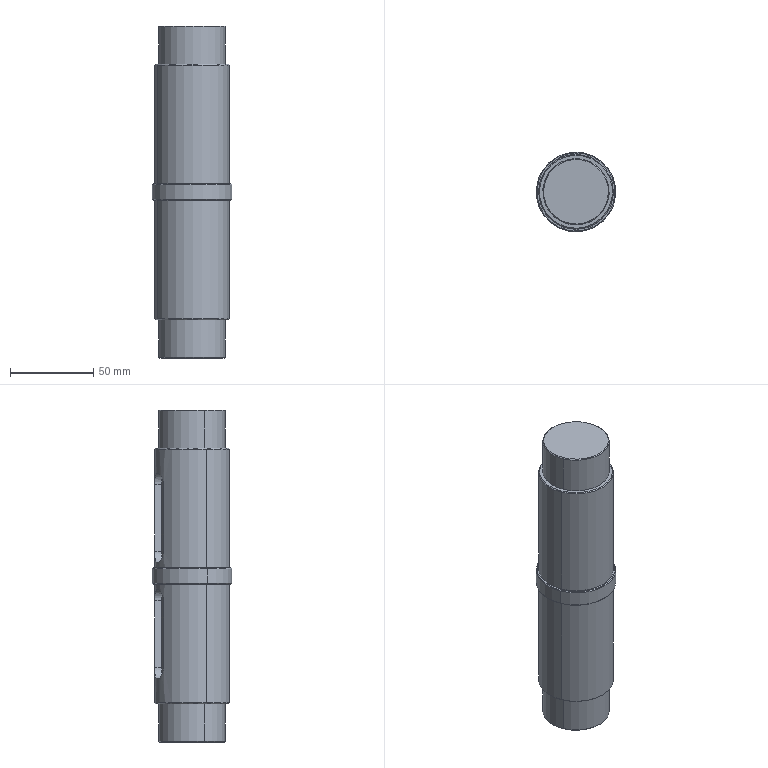Part | SolidWorks | features BaseBody 1 | 1 solid | 40 faces | box 48 x 48 x 200 mm | volume 297463 mm3 | cylinder 16 | cone 12 | plane 12 | commonest cylinder face diameters 14 x6 40 x4 45 x4 48 x2
STEP:
#1=CARTESIAN_POINT('',(446.784,55.988,-196.693));
#2=VERTEX_POINT('',#1);
#3=CARTESIAN_POINT('',(453.254,58.66,-203.693));
#4=VERTEX_POINT('',#3);
#5=CARTESIAN_POINT('',(446.784,55.988,-203.693));
#6=DIRECTION('',(-0.3818,0.9243,0.));
#7=DIRECTION('',(0.,0.,1.));
#8=AXIS2_PLACEMENT_3D('',#5,#6,#7);
#9=CIRCLE('',#8,7.);
#10=EDGE_CURVE('',#2,#4,#9,.T.);
#11=ORIENTED_EDGE('',*,*,#10,.F.);
#12=CARTESIAN_POINT('',(444.684,61.071,-196.693));
#13=VERTEX_POINT('',#12);
#14=CARTESIAN_POINT('',(446.784,55.988,-196.693));
#15=DIRECTION('',(-0.3818,0.9243,0.));
#16=VECTOR('',#15,1000.);
#17=LINE('',#14,#16);
#18=EDGE_CURVE('',#2,#13,#17,.T.);
#19=ORIENTED_EDGE('',*,*,#18,.T.);
#20=CARTESIAN_POINT('',(451.581,62.712,-203.693));
#21=VERTEX_POINT('',#20);
#22=CARTESIAN_POINT('',(451.581,62.712,-203.693));
#23=CARTESIAN_POINT('',(451.581,62.712,-203.227));
#24=CARTESIAN_POINT('',(451.532,62.708,-202.77));
#25=CARTESIAN_POINT('',(451.391,62.697,-202.096));
#26=CARTESIAN_POINT('',(451.333,62.692,-201.873));
#27=CARTESIAN_POINT('',(451.192,62.679,-201.432));
#28=CARTESIAN_POINT('',(451.11,62.672,-201.213));
#29=CARTESIAN_POINT('',(450.836,62.644,-200.578));
#30=CARTESIAN_POINT('',(450.613,62.619,-200.177));
#31=CARTESIAN_POINT('',(450.222,62.568,-199.608));
#32=CARTESIAN_POINT('',(450.081,62.548,-199.423));
#33=CARTESIAN_POINT('',(449.785,62.504,-199.07));
#34=CARTESIAN_POINT('',(449.63,62.479,-198.901));
#35=CARTESIAN_POINT('',(449.143,62.396,-198.421));
#36=CARTESIAN_POINT('',(448.792,62.328,-198.132));
#37=CARTESIAN_POINT('',(448.033,62.16,-197.62));
#38=CARTESIAN_POINT('',(447.638,62.062,-197.404));
#39=CARTESIAN_POINT('',(447.026,61.892,-197.142));
#40=CARTESIAN_POINT('',(446.818,61.831,-197.064));
#41=CARTESIAN_POINT('',(446.396,61.7,-196.93));
#42=CARTESIAN_POINT('',(446.18,61.629,-196.873));
#43=CARTESIAN_POINT('',(445.537,61.408,-196.738));
#44=CARTESIAN_POINT('',(445.11,61.247,-196.693));
#45=CARTESIAN_POINT('',(444.684,61.071,-196.693));
#46=B_SPLINE_CURVE_WITH_KNOTS('',3,(#22,#23,#24,#25,#26,#27,#28,#29,#30,#31,#32,#33,#34,#35,#36,#37,#38,#39,#40,#41,#42,#43,#44,#45),.UNSPECIFIED.,.F.,.F.,(4,2,2,2,2,2,2,2,2,2,2,4),(0.,0.001377,0.002065,0.002754,0.00413,0.004819,0.005507,0.006884,0.008261,0.008949,0.009637,0.01101),.UNSPECIFIED.);
#47=EDGE_CURVE('',#21,#13,#46,.T.);
#48=ORIENTED_EDGE('',*,*,#47,.F.);
#49=CARTESIAN_POINT('',(453.254,58.66,-203.693));
#50=DIRECTION('',(-0.3818,0.9243,0.));
#51=VECTOR('',#50,1000.);
#52=LINE('',#49,#51);
#53=EDGE_CURVE('',#4,#21,#52,.T.);
#54=ORIENTED_EDGE('',*,*,#53,.F.);
#55=EDGE_LOOP('',(#11,#19,#48,#54));
#56=FACE_OUTER_BOUND('',#55,.T.);
#57=CARTESIAN_POINT('',(446.784,55.988,-203.693));
#58=DIRECTION('',(-0.3818,0.9243,0.));
#59=DIRECTION('',(0.,0.,1.));
#60=AXIS2_PLACEMENT_3D('',#57,#58,#59);
#61=CYLINDRICAL_SURFACE('',#60,7.);
#62=ADVANCED_FACE('',(#56),#61,.F.);
#63=CARTESIAN_POINT('',(446.784,55.988,-266.693));
#64=VERTEX_POINT('',#63);
#65=CARTESIAN_POINT('',(453.254,58.66,-273.693));
#66=VERTEX_POINT('',#65);
#67=CARTESIAN_POINT('',(446.784,55.988,-273.693));
#68=DIRECTION('',(-0.3818,0.9243,0.));
#69=DIRECTION('',(0.,0.,1.));
#70=AXIS2_PLACEMENT_3D('',#67,#68,#69);
#71=CIRCLE('',#70,7.);
#72=EDGE_CURVE('',#64,#66,#71,.T.);
#73=ORIENTED_EDGE('',*,*,#72,.F.);
#74=CARTESIAN_POINT('',(444.684,61.071,-266.693));
#75=VERTEX_POINT('',#74);
#76=CARTESIAN_POINT('',(446.784,55.988,-266.693));
#77=DIRECTION('',(-0.3818,0.9243,0.));
#78=VECTOR('',#77,1000.);
#79=LINE('',#76,#78);
#80=EDGE_CURVE('',#64,#75,#79,.T.);
#81=ORIENTED_EDGE('',*,*,#80,.T.);
#82=CARTESIAN_POINT('',(451.581,62.712,-273.693));
#83=VERTEX_POINT('',#82);
#84=CARTESIAN_POINT('',(451.581,62.712,-273.693));
#85=CARTESIAN_POINT('',(451.581,62.712,-273.227));
#86=CARTESIAN_POINT('',(451.532,62.708,-272.77));
#87=CARTESIAN_POINT('',(451.391,62.697,-272.096));
#88=CARTESIAN_POINT('',(451.333,62.692,-271.873));
#89=CARTESIAN_POINT('',(451.192,62.679,-271.432));
#90=CARTESIAN_POINT('',(451.11,62.672,-271.213));
#91=CARTESIAN_POINT('',(450.836,62.644,-270.578));
#92=CARTESIAN_POINT('',(450.613,62.619,-270.177));
#93=CARTESIAN_POINT('',(450.222,62.568,-269.608));
#94=CARTESIAN_POINT('',(450.081,62.548,-269.423));
#95=CARTESIAN_POINT('',(449.785,62.504,-269.07));
#96=CARTESIAN_POINT('',(449.63,62.479,-268.901));
#97=CARTESIAN_POINT('',(449.143,62.396,-268.421));
#98=CARTESIAN_POINT('',(448.792,62.328,-268.132));
#99=CARTESIAN_POINT('',(448.033,62.16,-267.62));
#100=CARTESIAN_POINT('',(447.638,62.062,-267.404));
#101=CARTESIAN_POINT('',(447.026,61.892,-267.142));
#102=CARTESIAN_POINT('',(446.818,61.831,-267.064));
#103=CARTESIAN_POINT('',(446.396,61.7,-266.93));
#104=CARTESIAN_POINT('',(446.18,61.629,-266.873));
#105=CARTESIAN_POINT('',(445.537,61.408,-266.738));
#106=CARTESIAN_POINT('',(445.11,61.247,-266.693));
#107=CARTESIAN_POINT('',(444.684,61.071,-266.693));
#108=B_SPLINE_CURVE_WITH_KNOTS('',3,(#84,#85,#86,#87,#88,#89,#90,#91,#92,#93,#94,#95,#96,#97,#98,#99,#100,#101,#102,#103,#104,#105,#106,#107),.UNSPECIFIED.,.F.,.F.,(4,2,2,2,2,2,2,2,2,2,2,4),(0.,0.001377,0.002065,0.002754,0.00413,0.004819,0.005507,0.006884,0.008261,0.008949,0.009637,0.01101),.UNSPECIFIED.);
#109=EDGE_CURVE('',#83,#75,#108,.T.);
#110=ORIENTED_EDGE('',*,*,#109,.F.);
#111=CARTESIAN_POINT('',(453.254,58.66,-273.693));
#112=DIRECTION('',(-0.3818,0.9243,0.));
#113=VECTOR('',#112,1000.);
#114=LINE('',#111,#113);
#115=EDGE_CURVE('',#66,#83,#114,.T.);
#116=ORIENTED_EDGE('',*,*,#115,.F.);
#117=EDGE_LOOP('',(#73,#81,#110,#116));
#118=FACE_OUTER_BOUND('',#117,.T.);
#119=CARTESIAN_POINT('',(446.784,55.988,-273.693));
#120=DIRECTION('',(-0.3818,0.9243,0.));
#121=DIRECTION('',(0.,0.,1.));
#122=AXIS2_PLACEMENT_3D('',#119,#120,#121);
#123=CYLINDRICAL_SURFACE('',#122,7.);
#124=ADVANCED_FACE('',(#118),#123,.F.);
#125=CARTESIAN_POINT('',(473.608,48.675,-181.693));
#126=VERTEX_POINT('',#125);
#127=CARTESIAN_POINT('',(432.941,31.877,-181.693));
#128=VERTEX_POINT('',#127);
#129=CARTESIAN_POINT('',(453.274,40.276,-181.693));
#130=DIRECTION('',(0.,0.,1.));
#131=DIRECTION('',(0.9243,0.3818,0.));
#132=AXIS2_PLACEMENT_3D('',#129,#130,#131);
#133=CIRCLE('',#132,22.);
#134=EDGE_CURVE('',#126,#128,#133,.T.);
#135=ORIENTED_EDGE('',*,*,#134,.F.);
#136=CARTESIAN_POINT('',(474.07,48.865,-182.193));
#137=VERTEX_POINT('',#136);
#138=CARTESIAN_POINT('',(473.608,48.675,-181.693));
#139=DIRECTION('',(0.6535,0.27,-0.7071));
#140=VECTOR('',#139,1000.);
#141=LINE('',#138,#140);
#142=EDGE_CURVE('',#126,#137,#141,.T.);
#143=ORIENTED_EDGE('',*,*,#142,.T.);
#144=CARTESIAN_POINT('',(432.478,31.686,-182.193));
#145=VERTEX_POINT('',#144);
#146=CARTESIAN_POINT('',(453.274,40.276,-182.193));
#147=DIRECTION('',(0.,0.,-1.));
#148=DIRECTION('',(0.9243,0.3818,0.));
#149=AXIS2_PLACEMENT_3D('',#146,#147,#148);
#150=CIRCLE('',#149,22.5);
#151=EDGE_CURVE('',#145,#137,#150,.T.);
#152=ORIENTED_EDGE('',*,*,#151,.F.);
#153=CARTESIAN_POINT('',(432.941,31.877,-181.693));
#154=DIRECTION('',(-0.6535,-0.27,-0.7071));
#155=VECTOR('',#154,1000.);
#156=LINE('',#153,#155);
#157=EDGE_CURVE('',#128,#145,#156,.T.);
#158=ORIENTED_EDGE('',*,*,#157,.F.);
#159=EDGE_LOOP('',(#135,#143,#152,#158));
#160=FACE_OUTER_BOUND('',#159,.T.);
#161=CARTESIAN_POINT('',(453.274,40.276,-181.693));
#162=DIRECTION('',(0.,0.,-1.));
#163=DIRECTION('',(-0.9243,-0.3818,0.));
#164=AXIS2_PLACEMENT_3D('',#161,#162,#163);
#165=CONICAL_SURFACE('',#164,22.,0.7854);
#166=ADVANCED_FACE('',(#160),#165,.T.);
#167=CARTESIAN_POINT('',(471.297,47.72,-158.693));
#168=VERTEX_POINT('',#167);
#169=CARTESIAN_POINT('',(435.251,32.831,-158.693));
#170=VERTEX_POINT('',#169);
#171=CARTESIAN_POINT('',(453.274,40.276,-158.693));
#172=DIRECTION('',(0.,0.,1.));
#173=DIRECTION('',(0.9243,0.3818,0.));
#174=AXIS2_PLACEMENT_3D('',#171,#172,#173);
#175=CIRCLE('',#174,19.5);
#176=EDGE_CURVE('',#168,#170,#175,.T.);
#177=ORIENTED_EDGE('',*,*,#176,.F.);
#178=CARTESIAN_POINT('',(471.759,47.911,-159.193));
#179=VERTEX_POINT('',#178);
#180=CARTESIAN_POINT('',(471.297,47.72,-158.693));
#181=DIRECTION('',(0.6535,0.27,-0.7071));
#182=VECTOR('',#181,1000.);
#183=LINE('',#180,#182);
#184=EDGE_CURVE('',#168,#179,#183,.T.);
#185=ORIENTED_EDGE('',*,*,#184,.T.);
#186=CARTESIAN_POINT('',(434.789,32.64,-159.193));
#187=VERTEX_POINT('',#186);
#188=CARTESIAN_POINT('',(453.274,40.276,-159.193));
#189=DIRECTION('',(0.,0.,-1.));
#190=DIRECTION('',(0.9243,0.3818,0.));
#191=AXIS2_PLACEMENT_3D('',#188,#189,#190);
#192=CIRCLE('',#191,20.);
#193=EDGE_CURVE('',#187,#179,#192,.T.);
#194=ORIENTED_EDGE('',*,*,#193,.F.);
#195=CARTESIAN_POINT('',(435.251,32.831,-158.693));
#196=DIRECTION('',(-0.6535,-0.27,-0.7071));
#197=VECTOR('',#196,1000.);
#198=LINE('',#195,#197);
#199=EDGE_CURVE('',#170,#187,#198,.T.);
#200=ORIENTED_EDGE('',*,*,#199,.F.);
#201=EDGE_LOOP('',(#177,#185,#194,#200));
#202=FACE_OUTER_BOUND('',#201,.T.);
#203=CARTESIAN_POINT('',(453.274,40.276,-158.693));
#204=DIRECTION('',(0.,0.,-1.));
#205=DIRECTION('',(-0.9243,-0.3818,0.));
#206=AXIS2_PLACEMENT_3D('',#203,#204,#205);
#207=CONICAL_SURFACE('',#206,19.5,0.7854);
#208=ADVANCED_FACE('',(#202),#207,.T.);
#209=CARTESIAN_POINT('',(474.994,49.247,-253.693));
#210=VERTEX_POINT('',#209);
#211=CARTESIAN_POINT('',(431.554,31.304,-253.693));
#212=VERTEX_POINT('',#211);
#213=CARTESIAN_POINT('',(453.274,40.276,-253.693));
#214=DIRECTION('',(0.,0.,1.));
#215=DIRECTION('',(0.9243,0.3818,0.));
#216=AXIS2_PLACEMENT_3D('',#213,#214,#215);
#217=CIRCLE('',#216,23.5);
#218=EDGE_CURVE('',#210,#212,#217,.T.);
#219=ORIENTED_EDGE('',*,*,#218,.F.);
#220=CARTESIAN_POINT('',(475.456,49.438,-254.193));
#221=VERTEX_POINT('',#220);
#222=CARTESIAN_POINT('',(474.994,49.247,-253.693));
#223=DIRECTION('',(0.6535,0.27,-0.7071));
#224=VECTOR('',#223,1000.);
#225=LINE('',#222,#224);
#226=EDGE_CURVE('',#210,#221,#225,.T.);
#227=ORIENTED_EDGE('',*,*,#226,.T.);
#228=CARTESIAN_POINT('',(431.092,31.113,-254.193));
#229=VERTEX_POINT('',#228);
#230=CARTESIAN_POINT('',(453.274,40.276,-254.193));
#231=DIRECTION('',(0.,0.,-1.));
#232=DIRECTION('',(0.9243,0.3818,0.));
#233=AXIS2_PLACEMENT_3D('',#230,#231,#232);
#234=CIRCLE('',#233,24.);
#235=EDGE_CURVE('',#229,#221,#234,.T.);
#236=ORIENTED_EDGE('',*,*,#235,.F.);
#237=CARTESIAN_POINT('',(431.554,31.304,-253.693));
#238=DIRECTION('',(-0.6535,-0.27,-0.7071));
#239=VECTOR('',#238,1000.);
#240=LINE('',#237,#239);
#241=EDGE_CURVE('',#212,#229,#240,.T.);
#242=ORIENTED_EDGE('',*,*,#241,.F.);
#243=EDGE_LOOP('',(#219,#227,#236,#242));
#244=FACE_OUTER_BOUND('',#243,.T.);
#245=CARTESIAN_POINT('',(453.274,40.276,-253.693));
#246=DIRECTION('',(0.,0.,-1.));
#247=DIRECTION('',(-0.9243,-0.3818,0.));
#248=AXIS2_PLACEMENT_3D('',#245,#246,#247);
#249=CONICAL_SURFACE('',#248,23.5,0.7854);
#250=ADVANCED_FACE('',(#244),#249,.T.);
#251=CARTESIAN_POINT('',(431.554,31.304,-263.693));
#252=VERTEX_POINT('',#251);
#253=CARTESIAN_POINT('',(474.994,49.247,-263.693));
#254=VERTEX_POINT('',#253);
#255=CARTESIAN_POINT('',(453.274,40.276,-263.693));
#256=DIRECTION('',(0.,0.,-1.));
#257=DIRECTION('',(-0.9243,-0.3818,0.));
#258=AXIS2_PLACEMENT_3D('',#255,#256,#257);
#259=CIRCLE('',#258,23.5);
#260=EDGE_CURVE('',#252,#254,#259,.T.);
#261=ORIENTED_EDGE('',*,*,#260,.F.);
#262=CARTESIAN_POINT('',(431.092,31.113,-263.193));
#263=VERTEX_POINT('',#262);
#264=CARTESIAN_POINT('',(431.092,31.113,-263.193));
#265=DIRECTION('',(-0.6535,-0.27,0.7071));
#266=VECTOR('',#265,1000.);
#267=LINE('',#264,#266);
#268=EDGE_CURVE('',#252,#263,#267,.T.);
#269=ORIENTED_EDGE('',*,*,#268,.T.);
#270=CARTESIAN_POINT('',(475.456,49.438,-263.193));
#271=VERTEX_POINT('',#270);
#272=CARTESIAN_POINT('',(453.274,40.276,-263.193));
#273=DIRECTION('',(0.,0.,1.));
#274=DIRECTION('',(-0.9243,-0.3818,0.));
#275=AXIS2_PLACEMENT_3D('',#272,#273,#274);
#276=CIRCLE('',#275,24.);
#277=EDGE_CURVE('',#271,#263,#276,.T.);
#278=ORIENTED_EDGE('',*,*,#277,.F.);
#279=CARTESIAN_POINT('',(475.456,49.438,-263.193));
#280=DIRECTION('',(0.6535,0.27,0.7071));
#281=VECTOR('',#280,1000.);
#282=LINE('',#279,#281);
#283=EDGE_CURVE('',#254,#271,#282,.T.);
#284=ORIENTED_EDGE('',*,*,#283,.F.);
#285=EDGE_LOOP('',(#261,#269,#278,#284));
#286=FACE_OUTER_BOUND('',#285,.T.);
#287=CARTESIAN_POINT('',(453.274,40.276,-263.193));
#288=DIRECTION('',(0.,0.,1.));
#289=DIRECTION('',(0.9243,0.3818,0.));
#290=AXIS2_PLACEMENT_3D('',#287,#288,#289);
#291=CONICAL_SURFACE('',#290,24.,0.7854);
#292=ADVANCED_FACE('',(#286),#291,.T.);
#293=CARTESIAN_POINT('',(432.941,31.877,-335.693));
#294=VERTEX_POINT('',#293);
#295=CARTESIAN_POINT('',(473.608,48.675,-335.693));
#296=VERTEX_POINT('',#295);
#297=CARTESIAN_POINT('',(453.274,40.276,-335.693));
#298=DIRECTION('',(0.,0.,-1.));
#299=DIRECTION('',(0.9243,0.3818,0.));
#300=AXIS2_PLACEMENT_3D('',#297,#298,#299);
#301=CIRCLE('',#300,22.);
#302=EDGE_CURVE('',#294,#296,#301,.T.);
#303=ORIENTED_EDGE('',*,*,#302,.F.);
#304=CARTESIAN_POINT('',(432.478,31.686,-335.193));
#305=VERTEX_POINT('',#304);
#306=CARTESIAN_POINT('',(432.478,31.686,-335.193));
#307=DIRECTION('',(-0.6535,-0.27,0.7071));
#308=VECTOR('',#307,1000.);
#309=LINE('',#306,#308);
#310=EDGE_CURVE('',#294,#305,#309,.T.);
#311=ORIENTED_EDGE('',*,*,#310,.T.);
#312=CARTESIAN_POINT('',(474.07,48.865,-335.193));
#313=VERTEX_POINT('',#312);
#314=CARTESIAN_POINT('',(453.274,40.276,-335.193));
#315=DIRECTION('',(0.,0.,1.));
#316=DIRECTION('',(0.9243,0.3818,0.));
#317=AXIS2_PLACEMENT_3D('',#314,#315,#316);
#318=CIRCLE('',#317,22.5);
#319=EDGE_CURVE('',#313,#305,#318,.T.);
#320=ORIENTED_EDGE('',*,*,#319,.F.);
#321=CARTESIAN_POINT('',(474.07,48.865,-335.193));
#322=DIRECTION('',(0.6535,0.27,0.7071));
#323=VECTOR('',#322,1000.);
#324=LINE('',#321,#323);
#325=EDGE_CURVE('',#296,#313,#324,.T.);
#326=ORIENTED_EDGE('',*,*,#325,.F.);
#327=EDGE_LOOP('',(#303,#311,#320,#326));
#328=FACE_OUTER_BOUND('',#327,.T.);
#329=CARTESIAN_POINT('',(453.274,40.276,-335.193));
#330=DIRECTION('',(0.,0.,1.));
#331=DIRECTION('',(0.9243,0.3818,0.));
#332=AXIS2_PLACEMENT_3D('',#329,#330,#331);
#333=CONICAL_SURFACE('',#332,22.5,0.7854);
#334=ADVANCED_FACE('',(#328),#333,.T.);
#335=CARTESIAN_POINT('',(435.251,32.831,-358.693));
#336=VERTEX_POINT('',#335);
#337=CARTESIAN_POINT('',(471.297,47.72,-358.693));
#338=VERTEX_POINT('',#337);
#339=CARTESIAN_POINT('',(453.274,40.276,-358.693));
#340=DIRECTION('',(0.,0.,-1.));
#341=DIRECTION('',(-0.9243,-0.3818,0.));
#342=AXIS2_PLACEMENT_3D('',#339,#340,#341);
#343=CIRCLE('',#342,19.5);
#344=EDGE_CURVE('',#336,#338,#343,.T.);
#345=ORIENTED_EDGE('',*,*,#344,.F.);
#346=CARTESIAN_POINT('',(434.789,32.64,-358.193));
#347=VERTEX_POINT('',#346);
#348=CARTESIAN_POINT('',(435.251,32.831,-358.693));
#349=DIRECTION('',(-0.6535,-0.27,0.7071));
#350=VECTOR('',#349,1000.);
#351=LINE('',#348,#350);
#352=EDGE_CURVE('',#336,#347,#351,.T.);
#353=ORIENTED_EDGE('',*,*,#352,.T.);
#354=CARTESIAN_POINT('',(471.759,47.911,-358.193));
#355=VERTEX_POINT('',#354);
#356=CARTESIAN_POINT('',(453.274,40.276,-358.193));
#357=DIRECTION('',(0.,0.,1.));
#358=DIRECTION('',(-0.9243,-0.3818,0.));
#359=AXIS2_PLACEMENT_3D('',#356,#357,#358);
#360=CIRCLE('',#359,20.);
#361=EDGE_CURVE('',#355,#347,#360,.T.);
#362=ORIENTED_EDGE('',*,*,#361,.F.);
#363=CARTESIAN_POINT('',(471.297,47.72,-358.693));
#364=DIRECTION('',(0.6535,0.27,0.7071));
#365=VECTOR('',#364,1000.);
#366=LINE('',#363,#365);
#367=EDGE_CURVE('',#338,#355,#366,.T.);
#368=ORIENTED_EDGE('',*,*,#367,.F.);
#369=EDGE_LOOP('',(#345,#353,#362,#368));
#370=FACE_OUTER_BOUND('',#369,.T.);
#371=CARTESIAN_POINT('',(453.274,40.276,-358.693));
#372=DIRECTION('',(0.,0.,1.));
#373=DIRECTION('',(0.9243,0.3818,0.));
#374=AXIS2_PLACEMENT_3D('',#371,#372,#373);
#375=CONICAL_SURFACE('',#374,19.5,0.7854);
#376=ADVANCED_FACE('',(#370),#375,.T.);
#377=ORIENTED_EDGE('',*,*,#361,.T.);
#378=CARTESIAN_POINT('',(434.789,32.64,-335.693));
#379=VERTEX_POINT('',#378);
#380=CARTESIAN_POINT('',(434.789,32.64,-358.693));
#381=DIRECTION('',(0.,0.,1.));
#382=VECTOR('',#381,1000.);
#383=LINE('',#380,#382);
#384=EDGE_CURVE('',#347,#379,#383,.T.);
#385=ORIENTED_EDGE('',*,*,#384,.T.);
#386=CARTESIAN_POINT('',(471.759,47.911,-335.693));
#387=VERTEX_POINT('',#386);
#388=CARTESIAN_POINT('',(453.274,40.276,-335.693));
#389=DIRECTION('',(0.,0.,-1.));
#390=DIRECTION('',(0.9243,0.3818,0.));
#391=AXIS2_PLACEMENT_3D('',#388,#389,#390);
#392=CIRCLE('',#391,20.);
#393=EDGE_CURVE('',#379,#387,#392,.T.);
#394=ORIENTED_EDGE('',*,*,#393,.T.);
#395=CARTESIAN_POINT('',(471.759,47.911,-358.693));
#396=DIRECTION('',(0.,0.,1.));
#397=VECTOR('',#396,1000.);
#398=LINE('',#395,#397);
#399=EDGE_CURVE('',#355,#387,#398,.T.);
#400=ORIENTED_EDGE('',*,*,#399,.F.);
#401=EDGE_LOOP('',(#377,#385,#394,#400));
#402=FACE_OUTER_BOUND('',#401,.T.);
#403=CARTESIAN_POINT('',(453.274,40.276,-358.693));
#404=DIRECTION('',(0.,0.,1.));
#405=DIRECTION('',(0.9243,0.3818,0.));
#406=AXIS2_PLACEMENT_3D('',#403,#404,#405);
#407=CYLINDRICAL_SURFACE('',#406,20.);
#408=ADVANCED_FACE('',(#402),#407,.T.);
#409=ORIENTED_EDGE('',*,*,#193,.T.);
#410=CARTESIAN_POINT('',(471.759,47.911,-181.693));
#411=VERTEX_POINT('',#410);
#412=CARTESIAN_POINT('',(471.759,47.911,-158.693));
#413=DIRECTION('',(0.,0.,-1.));
#414=VECTOR('',#413,1000.);
#415=LINE('',#412,#414);
#416=EDGE_CURVE('',#179,#411,#415,.T.);
#417=ORIENTED_EDGE('',*,*,#416,.T.);
#418=CARTESIAN_POINT('',(434.789,32.64,-181.693));
#419=VERTEX_POINT('',#418);
#420=CARTESIAN_POINT('',(453.274,40.276,-181.693));
#421=DIRECTION('',(0.,0.,1.));
#422=DIRECTION('',(0.9243,0.3818,0.));
#423=AXIS2_PLACEMENT_3D('',#420,#421,#422);
#424=CIRCLE('',#423,20.);
#425=EDGE_CURVE('',#411,#419,#424,.T.);
#426=ORIENTED_EDGE('',*,*,#425,.T.);
#427=CARTESIAN_POINT('',(434.789,32.64,-158.693));
#428=DIRECTION('',(0.,0.,-1.));
#429=VECTOR('',#428,1000.);
#430=LINE('',#427,#429);
#431=EDGE_CURVE('',#187,#419,#430,.T.);
#432=ORIENTED_EDGE('',*,*,#431,.F.);
#433=EDGE_LOOP('',(#409,#417,#426,#432));
#434=FACE_OUTER_BOUND('',#433,.T.);
#435=CARTESIAN_POINT('',(453.274,40.276,-158.693));
#436=DIRECTION('',(0.,0.,-1.));
#437=DIRECTION('',(-0.9243,-0.3818,0.));
#438=AXIS2_PLACEMENT_3D('',#435,#436,#437);
#439=CYLINDRICAL_SURFACE('',#438,20.);
#440=ADVANCED_FACE('',(#434),#439,.T.);
#441=CARTESIAN_POINT('',(438.641,57.367,-273.693));
#442=VERTEX_POINT('',#441);
#443=CARTESIAN_POINT('',(438.641,57.367,-313.693));
#444=VERTEX_POINT('',#443);
#445=CARTESIAN_POINT('',(438.641,57.367,-181.693));
#446=DIRECTION('',(0.,0.,-1.));
#447=VECTOR('',#446,1000.);
#448=LINE('',#445,#447);
#449=EDGE_CURVE('',#442,#444,#448,.T.);
#450=ORIENTED_EDGE('',*,*,#449,.T.);
#451=CARTESIAN_POINT('',(451.581,62.712,-313.693));
#452=VERTEX_POINT('',#451);
#453=CARTESIAN_POINT('',(438.641,57.367,-313.693));
#454=CARTESIAN_POINT('',(438.641,57.367,-314.158));
#455=CARTESIAN_POINT('',(438.678,57.399,-314.616));
#456=CARTESIAN_POINT('',(438.786,57.49,-315.289));
#457=CARTESIAN_POINT('',(438.83,57.528,-315.512));
#458=CARTESIAN_POINT('',(438.939,57.618,-315.953));
#459=CARTESIAN_POINT('',(439.002,57.67,-316.171));
#460=CARTESIAN_POINT('',(439.216,57.844,-316.806));
#461=CARTESIAN_POINT('',(439.391,57.984,-317.207));
#462=CARTESIAN_POINT('',(439.704,58.223,-317.775));
#463=CARTESIAN_POINT('',(439.817,58.308,-317.961));
#464=CARTESIAN_POINT('',(440.058,58.486,-318.314));
#465=CARTESIAN_POINT('',(440.185,58.578,-318.482));
#466=CARTESIAN_POINT('',(440.588,58.861,-318.963));
#467=CARTESIAN_POINT('',(440.885,59.061,-319.252));
#468=CARTESIAN_POINT('',(441.54,59.477,-319.764));
#469=CARTESIAN_POINT('',(441.889,59.687,-319.979));
#470=CARTESIAN_POINT('',(442.442,59.998,-320.242));
#471=CARTESIAN_POINT('',(442.632,60.101,-320.32));
#472=CARTESIAN_POINT('',(443.023,60.306,-320.454));
#473=CARTESIAN_POINT('',(443.226,60.408,-320.511));
#474=CARTESIAN_POINT('',(443.837,60.706,-320.647));
#475=CARTESIAN_POINT('',(444.253,60.893,-320.693));
#476=CARTESIAN_POINT('',(445.103,61.244,-320.693));
#477=CARTESIAN_POINT('',(445.54,61.409,-320.647));
#478=CARTESIAN_POINT('',(446.393,61.702,-320.468));
#479=CARTESIAN_POINT('',(446.813,61.832,-320.335));
#480=CARTESIAN_POINT('',(447.432,62.005,-320.07));
#481=CARTESIAN_POINT('',(447.636,62.059,-319.971));
#482=CARTESIAN_POINT('',(448.031,62.157,-319.755));
#483=CARTESIAN_POINT('',(448.224,62.202,-319.638));
#484=CARTESIAN_POINT('',(448.598,62.285,-319.385));
#485=CARTESIAN_POINT('',(448.78,62.323,-319.25));
#486=CARTESIAN_POINT('',(449.133,62.392,-318.96));
#487=CARTESIAN_POINT('',(449.305,62.423,-318.805));
#488=CARTESIAN_POINT('',(449.794,62.507,-318.322));
#489=CARTESIAN_POINT('',(450.088,62.55,-317.972));
#490=CARTESIAN_POINT('',(450.608,62.619,-317.216));
#491=CARTESIAN_POINT('',(450.836,62.644,-316.807));
#492=CARTESIAN_POINT('',(451.201,62.681,-315.964));
#493=CARTESIAN_POINT('',(451.341,62.693,-315.528));
#494=CARTESIAN_POINT('',(451.484,62.704,-314.85));
#495=CARTESIAN_POINT('',(451.52,62.707,-314.619));
#496=CARTESIAN_POINT('',(451.568,62.711,-314.158));
#497=CARTESIAN_POINT('',(451.581,62.712,-313.926));
#498=CARTESIAN_POINT('',(451.581,62.712,-313.693));
#499=B_SPLINE_CURVE_WITH_KNOTS('',3,(#453,#454,#455,#456,#457,#458,#459,#460,#461,#462,#463,#464,#465,#466,#467,#468,#469,#470,#471,#472,#473,#474,#475,#476,#477,#478,#479,#480,#481,#482,#483,#484,#485,#486,#487,#488,#489,#490,#491,#492,#493,#494,#495,#496,#497,#498),.UNSPECIFIED.,.F.,.F.,(4,2,2,2,2,2,2,2,2,2,2,2,2,2,2,2,2,2,2,2,2,2,4),(0.,0.001376,0.002064,0.002752,0.004128,0.004816,0.005504,0.006879,0.008255,0.008943,0.009631,0.01101,0.01238,0.01376,0.01445,0.01513,0.01582,0.01651,0.01789,0.01926,0.02064,0.02133,0.02201),.UNSPECIFIED.);
#500=EDGE_CURVE('',#444,#452,#499,.T.);
#501=ORIENTED_EDGE('',*,*,#500,.T.);
#502=CARTESIAN_POINT('',(451.581,62.712,-181.693));
#503=DIRECTION('',(0.,0.,1.));
#504=VECTOR('',#503,1000.);
#505=LINE('',#502,#504);
#506=EDGE_CURVE('',#452,#83,#505,.T.);
#507=ORIENTED_EDGE('',*,*,#506,.T.);
#508=ORIENTED_EDGE('',*,*,#109,.T.);
#509=CARTESIAN_POINT('',(444.684,61.071,-266.693));
#510=CARTESIAN_POINT('',(444.26,60.896,-266.693));
#511=CARTESIAN_POINT('',(443.834,60.704,-266.739));
#512=CARTESIAN_POINT('',(443.024,60.31,-266.92));
#513=CARTESIAN_POINT('',(442.635,60.106,-267.053));
#514=CARTESIAN_POINT('',(442.075,59.791,-267.318));
#515=CARTESIAN_POINT('',(441.893,59.686,-267.417));
#516=CARTESIAN_POINT('',(441.544,59.477,-267.633));
#517=CARTESIAN_POINT('',(441.376,59.373,-267.751));
#518=CARTESIAN_POINT('',(441.052,59.168,-268.003));
#519=CARTESIAN_POINT('',(440.897,59.066,-268.139));
#520=CARTESIAN_POINT('',(440.598,58.866,-268.428));
#521=CARTESIAN_POINT('',(440.454,58.767,-268.583));
#522=CARTESIAN_POINT('',(440.049,58.481,-269.067));
#523=CARTESIAN_POINT('',(439.811,58.305,-269.417));
#524=CARTESIAN_POINT('',(439.394,57.986,-270.172));
#525=CARTESIAN_POINT('',(439.216,57.844,-270.581));
#526=CARTESIAN_POINT('',(438.932,57.613,-271.423));
#527=CARTESIAN_POINT('',(438.824,57.523,-271.859));
#528=CARTESIAN_POINT('',(438.715,57.43,-272.537));
#529=CARTESIAN_POINT('',(438.687,57.406,-272.767));
#530=CARTESIAN_POINT('',(438.65,57.375,-273.229));
#531=CARTESIAN_POINT('',(438.641,57.367,-273.46));
#532=CARTESIAN_POINT('',(438.641,57.367,-273.693));
#533=B_SPLINE_CURVE_WITH_KNOTS('',3,(#509,#510,#511,#512,#513,#514,#515,#516,#517,#518,#519,#520,#521,#522,#523,#524,#525,#526,#527,#528,#529,#530,#531,#532),.UNSPECIFIED.,.F.,.F.,(4,2,2,2,2,2,2,2,2,2,2,4),(0.01101,0.01239,0.01376,0.01445,0.01514,0.01583,0.01651,0.01789,0.01926,0.02064,0.02133,0.02201),.UNSPECIFIED.);
#534=EDGE_CURVE('',#75,#442,#533,.T.);
#535=ORIENTED_EDGE('',*,*,#534,.T.);
#536=EDGE_LOOP('',(#450,#501,#507,#508,#535));
#537=FACE_BOUND('',#536,.T.);
#538=CARTESIAN_POINT('',(432.478,31.686,-263.693));
#539=VERTEX_POINT('',#538);
#540=CARTESIAN_POINT('',(474.07,48.865,-263.693));
#541=VERTEX_POINT('',#540);
#542=CARTESIAN_POINT('',(453.274,40.276,-263.693));
#543=DIRECTION('',(0.,0.,-1.));
#544=DIRECTION('',(-0.9243,-0.3818,0.));
#545=AXIS2_PLACEMENT_3D('',#542,#543,#544);
#546=CIRCLE('',#545,22.5);
#547=EDGE_CURVE('',#539,#541,#546,.T.);
#548=ORIENTED_EDGE('',*,*,#547,.T.);
#549=CARTESIAN_POINT('',(474.07,48.865,-181.693));
#550=DIRECTION('',(0.,0.,-1.));
#551=VECTOR('',#550,1000.);
#552=LINE('',#549,#551);
#553=EDGE_CURVE('',#541,#313,#552,.T.);
#554=ORIENTED_EDGE('',*,*,#553,.T.);
#555=ORIENTED_EDGE('',*,*,#319,.T.);
#556=CARTESIAN_POINT('',(432.478,31.686,-181.693));
#557=DIRECTION('',(0.,0.,-1.));
#558=VECTOR('',#557,1000.);
#559=LINE('',#556,#558);
#560=EDGE_CURVE('',#539,#305,#559,.T.);
#561=ORIENTED_EDGE('',*,*,#560,.F.);
#562=EDGE_LOOP('',(#548,#554,#555,#561));
#563=FACE_OUTER_BOUND('',#562,.T.);
#564=CARTESIAN_POINT('',(453.274,40.276,-181.693));
#565=DIRECTION('',(0.,0.,-1.));
#566=DIRECTION('',(-0.9243,-0.3818,0.));
#567=AXIS2_PLACEMENT_3D('',#564,#565,#566);
#568=CYLINDRICAL_SURFACE('',#567,22.5);
#569=ADVANCED_FACE('',(#537,#563),#568,.T.);
#570=ORIENTED_EDGE('',*,*,#235,.T.);
#571=CARTESIAN_POINT('',(475.456,49.438,-253.693));
#572=DIRECTION('',(0.,0.,-1.));
#573=VECTOR('',#572,1000.);
#574=LINE('',#571,#573);
#575=EDGE_CURVE('',#221,#271,#574,.T.);
#576=ORIENTED_EDGE('',*,*,#575,.T.);
#577=ORIENTED_EDGE('',*,*,#277,.T.);
#578=CARTESIAN_POINT('',(431.092,31.113,-253.693));
#579=DIRECTION('',(0.,0.,-1.));
#580=VECTOR('',#579,1000.);
#581=LINE('',#578,#580);
#582=EDGE_CURVE('',#229,#263,#581,.T.);
#583=ORIENTED_EDGE('',*,*,#582,.F.);
#584=EDGE_LOOP('',(#570,#576,#577,#583));
#585=FACE_OUTER_BOUND('',#584,.T.);
#586=CARTESIAN_POINT('',(453.274,40.276,-253.693));
#587=DIRECTION('',(0.,0.,-1.));
#588=DIRECTION('',(-0.9243,-0.3818,0.));
#589=AXIS2_PLACEMENT_3D('',#586,#587,#588);
#590=CYLINDRICAL_SURFACE('',#589,24.);
#591=ADVANCED_FACE('',(#585),#590,.T.);
#592=CARTESIAN_POINT('',(438.641,57.367,-203.693));
#593=VERTEX_POINT('',#592);
#594=CARTESIAN_POINT('',(438.641,57.367,-243.693));
#595=VERTEX_POINT('',#594);
#596=CARTESIAN_POINT('',(438.641,57.367,-181.693));
#597=DIRECTION('',(0.,0.,-1.));
#598=VECTOR('',#597,1000.);
#599=LINE('',#596,#598);
#600=EDGE_CURVE('',#593,#595,#599,.T.);
#601=ORIENTED_EDGE('',*,*,#600,.T.);
#602=CARTESIAN_POINT('',(451.581,62.712,-243.693));
#603=VERTEX_POINT('',#602);
#604=CARTESIAN_POINT('',(438.641,57.367,-243.693));
#605=CARTESIAN_POINT('',(438.641,57.367,-244.158));
#606=CARTESIAN_POINT('',(438.678,57.399,-244.616));
#607=CARTESIAN_POINT('',(438.786,57.49,-245.289));
#608=CARTESIAN_POINT('',(438.83,57.528,-245.512));
#609=CARTESIAN_POINT('',(438.939,57.618,-245.953));
#610=CARTESIAN_POINT('',(439.002,57.67,-246.171));
#611=CARTESIAN_POINT('',(439.216,57.844,-246.806));
#612=CARTESIAN_POINT('',(439.391,57.984,-247.207));
#613=CARTESIAN_POINT('',(439.704,58.223,-247.775));
#614=CARTESIAN_POINT('',(439.817,58.308,-247.961));
#615=CARTESIAN_POINT('',(440.058,58.486,-248.314));
#616=CARTESIAN_POINT('',(440.185,58.578,-248.482));
#617=CARTESIAN_POINT('',(440.588,58.861,-248.963));
#618=CARTESIAN_POINT('',(440.885,59.061,-249.252));
#619=CARTESIAN_POINT('',(441.54,59.477,-249.764));
#620=CARTESIAN_POINT('',(441.889,59.687,-249.979));
#621=CARTESIAN_POINT('',(442.442,59.998,-250.242));
#622=CARTESIAN_POINT('',(442.632,60.101,-250.32));
#623=CARTESIAN_POINT('',(443.023,60.306,-250.454));
#624=CARTESIAN_POINT('',(443.226,60.408,-250.511));
#625=CARTESIAN_POINT('',(443.837,60.706,-250.647));
#626=CARTESIAN_POINT('',(444.253,60.893,-250.693));
#627=CARTESIAN_POINT('',(445.103,61.244,-250.693));
#628=CARTESIAN_POINT('',(445.54,61.409,-250.647));
#629=CARTESIAN_POINT('',(446.393,61.702,-250.468));
#630=CARTESIAN_POINT('',(446.813,61.832,-250.335));
#631=CARTESIAN_POINT('',(447.432,62.005,-250.07));
#632=CARTESIAN_POINT('',(447.636,62.059,-249.971));
#633=CARTESIAN_POINT('',(448.031,62.157,-249.755));
#634=CARTESIAN_POINT('',(448.224,62.202,-249.638));
#635=CARTESIAN_POINT('',(448.598,62.285,-249.385));
#636=CARTESIAN_POINT('',(448.78,62.323,-249.25));
#637=CARTESIAN_POINT('',(449.133,62.392,-248.96));
#638=CARTESIAN_POINT('',(449.305,62.423,-248.805));
#639=CARTESIAN_POINT('',(449.794,62.507,-248.322));
#640=CARTESIAN_POINT('',(450.088,62.55,-247.972));
#641=CARTESIAN_POINT('',(450.608,62.619,-247.216));
#642=CARTESIAN_POINT('',(450.836,62.644,-246.807));
#643=CARTESIAN_POINT('',(451.201,62.681,-245.964));
#644=CARTESIAN_POINT('',(451.341,62.693,-245.528));
#645=CARTESIAN_POINT('',(451.484,62.704,-244.85));
#646=CARTESIAN_POINT('',(451.52,62.707,-244.619));
#647=CARTESIAN_POINT('',(451.568,62.711,-244.158));
#648=CARTESIAN_POINT('',(451.581,62.712,-243.926));
#649=CARTESIAN_POINT('',(451.581,62.712,-243.693));
#650=B_SPLINE_CURVE_WITH_KNOTS('',3,(#604,#605,#606,#607,#608,#609,#610,#611,#612,#613,#614,#615,#616,#617,#618,#619,#620,#621,#622,#623,#624,#625,#626,#627,#628,#629,#630,#631,#632,#633,#634,#635,#636,#637,#638,#639,#640,#641,#642,#643,#644,#645,#646,#647,#648,#649),.UNSPECIFIED.,.F.,.F.,(4,2,2,2,2,2,2,2,2,2,2,2,2,2,2,2,2,2,2,2,2,2,4),(0.,0.001376,0.002064,0.002752,0.004128,0.004816,0.005504,0.006879,0.008255,0.008943,0.009631,0.01101,0.01238,0.01376,0.01445,0.01513,0.01582,0.01651,0.01789,0.01926,0.02064,0.02133,0.02201),.UNSPECIFIED.);
#651=EDGE_CURVE('',#595,#603,#650,.T.);
#652=ORIENTED_EDGE('',*,*,#651,.T.);
#653=CARTESIAN_POINT('',(451.581,62.712,-181.693));
#654=DIRECTION('',(0.,0.,1.));
#655=VECTOR('',#654,1000.);
#656=LINE('',#653,#655);
#657=EDGE_CURVE('',#603,#21,#656,.T.);
#658=ORIENTED_EDGE('',*,*,#657,.T.);
#659=ORIENTED_EDGE('',*,*,#47,.T.);
#660=CARTESIAN_POINT('',(444.684,61.071,-196.693));
#661=CARTESIAN_POINT('',(444.26,60.896,-196.693));
#662=CARTESIAN_POINT('',(443.834,60.704,-196.739));
#663=CARTESIAN_POINT('',(443.024,60.31,-196.92));
#664=CARTESIAN_POINT('',(442.635,60.106,-197.053));
#665=CARTESIAN_POINT('',(442.075,59.791,-197.318));
#666=CARTESIAN_POINT('',(441.893,59.686,-197.417));
#667=CARTESIAN_POINT('',(441.544,59.477,-197.633));
#668=CARTESIAN_POINT('',(441.376,59.373,-197.751));
#669=CARTESIAN_POINT('',(441.052,59.168,-198.003));
#670=CARTESIAN_POINT('',(440.897,59.066,-198.139));
#671=CARTESIAN_POINT('',(440.598,58.866,-198.428));
#672=CARTESIAN_POINT('',(440.454,58.767,-198.583));
#673=CARTESIAN_POINT('',(440.049,58.481,-199.067));
#674=CARTESIAN_POINT('',(439.811,58.305,-199.417));
#675=CARTESIAN_POINT('',(439.394,57.986,-200.172));
#676=CARTESIAN_POINT('',(439.216,57.844,-200.581));
#677=CARTESIAN_POINT('',(438.932,57.613,-201.423));
#678=CARTESIAN_POINT('',(438.824,57.523,-201.859));
#679=CARTESIAN_POINT('',(438.715,57.43,-202.537));
#680=CARTESIAN_POINT('',(438.687,57.406,-202.767));
#681=CARTESIAN_POINT('',(438.65,57.375,-203.229));
#682=CARTESIAN_POINT('',(438.641,57.367,-203.46));
#683=CARTESIAN_POINT('',(438.641,57.367,-203.693));
#684=B_SPLINE_CURVE_WITH_KNOTS('',3,(#660,#661,#662,#663,#664,#665,#666,#667,#668,#669,#670,#671,#672,#673,#674,#675,#676,#677,#678,#679,#680,#681,#682,#683),.UNSPECIFIED.,.F.,.F.,(4,2,2,2,2,2,2,2,2,2,2,4),(0.01101,0.01239,0.01376,0.01445,0.01514,0.01583,0.01651,0.01789,0.01926,0.02064,0.02133,0.02201),.UNSPECIFIED.);
#685=EDGE_CURVE('',#13,#593,#684,.T.);
#686=ORIENTED_EDGE('',*,*,#685,.T.);
#687=EDGE_LOOP('',(#601,#652,#658,#659,#686));
#688=FACE_BOUND('',#687,.T.);
#689=ORIENTED_EDGE('',*,*,#151,.T.);
#690=CARTESIAN_POINT('',(474.07,48.865,-253.693));
#691=VERTEX_POINT('',#690);
#692=CARTESIAN_POINT('',(474.07,48.865,-181.693));
#693=DIRECTION('',(0.,0.,-1.));
#694=VECTOR('',#693,1000.);
#695=LINE('',#692,#694);
#696=EDGE_CURVE('',#137,#691,#695,.T.);
#697=ORIENTED_EDGE('',*,*,#696,.T.);
#698=CARTESIAN_POINT('',(432.478,31.686,-253.693));
#699=VERTEX_POINT('',#698);
#700=CARTESIAN_POINT('',(453.274,40.276,-253.693));
#701=DIRECTION('',(0.,0.,1.));
#702=DIRECTION('',(0.9243,0.3818,0.));
#703=AXIS2_PLACEMENT_3D('',#700,#701,#702);
#704=CIRCLE('',#703,22.5);
#705=EDGE_CURVE('',#691,#699,#704,.T.);
#706=ORIENTED_EDGE('',*,*,#705,.T.);
#707=CARTESIAN_POINT('',(432.478,31.686,-181.693));
#708=DIRECTION('',(0.,0.,-1.));
#709=VECTOR('',#708,1000.);
#710=LINE('',#707,#709);
#711=EDGE_CURVE('',#145,#699,#710,.T.);
#712=ORIENTED_EDGE('',*,*,#711,.F.);
#713=EDGE_LOOP('',(#689,#697,#706,#712));
#714=FACE_OUTER_BOUND('',#713,.T.);
#715=CARTESIAN_POINT('',(453.274,40.276,-181.693));
#716=DIRECTION('',(0.,0.,-1.));
#717=DIRECTION('',(-0.9243,-0.3818,0.));
#718=AXIS2_PLACEMENT_3D('',#715,#716,#717);
#719=CYLINDRICAL_SURFACE('',#718,22.5);
#720=ADVANCED_FACE('',(#688,#714),#719,.T.);
#721=ORIENTED_EDGE('',*,*,#696,.F.);
#722=CARTESIAN_POINT('',(453.274,40.276,-182.193));
#723=DIRECTION('',(0.,0.,-1.));
#724=DIRECTION('',(0.9243,0.3818,0.));
#725=AXIS2_PLACEMENT_3D('',#722,#723,#724);
#726=CIRCLE('',#725,22.5);
#727=EDGE_CURVE('',#137,#145,#726,.T.);
#728=ORIENTED_EDGE('',*,*,#727,.T.);
#729=ORIENTED_EDGE('',*,*,#711,.T.);
#730=CARTESIAN_POINT('',(453.274,40.276,-253.693));
#731=DIRECTION('',(0.,0.,1.));
#732=DIRECTION('',(0.9243,0.3818,0.));
#733=AXIS2_PLACEMENT_3D('',#730,#731,#732);
#734=CIRCLE('',#733,22.5);
#735=EDGE_CURVE('',#699,#691,#734,.T.);
#736=ORIENTED_EDGE('',*,*,#735,.T.);
#737=EDGE_LOOP('',(#721,#728,#729,#736));
#738=FACE_OUTER_BOUND('',#737,.T.);
#739=CARTESIAN_POINT('',(453.274,40.276,-181.693));
#740=DIRECTION('',(0.,0.,-1.));
#741=DIRECTION('',(-0.9243,-0.3818,0.));
#742=AXIS2_PLACEMENT_3D('',#739,#740,#741);
#743=CYLINDRICAL_SURFACE('',#742,22.5);
#744=ADVANCED_FACE('',(#738),#743,.T.);
#745=CARTESIAN_POINT('',(453.274,40.276,-181.693));
#746=DIRECTION('',(0.,0.,1.));
#747=DIRECTION('',(0.9243,0.3818,0.));
#748=AXIS2_PLACEMENT_3D('',#745,#746,#747);
#749=CIRCLE('',#748,22.);
#750=EDGE_CURVE('',#128,#126,#749,.T.);
#751=ORIENTED_EDGE('',*,*,#750,.T.);
#752=ORIENTED_EDGE('',*,*,#134,.T.);
#753=EDGE_LOOP('',(#751,#752));
#754=FACE_OUTER_BOUND('',#753,.T.);
#755=CARTESIAN_POINT('',(453.274,40.276,-181.693));
#756=DIRECTION('',(0.,0.,1.));
#757=DIRECTION('',(0.9243,0.3818,0.));
#758=AXIS2_PLACEMENT_3D('',#755,#756,#757);
#759=CIRCLE('',#758,20.);
#760=EDGE_CURVE('',#419,#411,#759,.T.);
#761=ORIENTED_EDGE('',*,*,#760,.F.);
#762=ORIENTED_EDGE('',*,*,#425,.F.);
#763=EDGE_LOOP('',(#761,#762));
#764=FACE_BOUND('',#763,.T.);
#765=CARTESIAN_POINT('',(453.274,40.276,-181.693));
#766=DIRECTION('',(0.,0.,1.));
#767=DIRECTION('',(0.9243,0.3818,0.));
#768=AXIS2_PLACEMENT_3D('',#765,#766,#767);
#769=PLANE('',#768);
#770=ADVANCED_FACE('',(#754,#764),#769,.T.);
#771=ORIENTED_EDGE('',*,*,#575,.F.);
#772=CARTESIAN_POINT('',(453.274,40.276,-254.193));
#773=DIRECTION('',(0.,0.,-1.));
#774=DIRECTION('',(0.9243,0.3818,0.));
#775=AXIS2_PLACEMENT_3D('',#772,#773,#774);
#776=CIRCLE('',#775,24.);
#777=EDGE_CURVE('',#221,#229,#776,.T.);
#778=ORIENTED_EDGE('',*,*,#777,.T.);
#779=ORIENTED_EDGE('',*,*,#582,.T.);
#780=CARTESIAN_POINT('',(453.274,40.276,-263.193));
#781=DIRECTION('',(0.,0.,1.));
#782=DIRECTION('',(-0.9243,-0.3818,0.));
#783=AXIS2_PLACEMENT_3D('',#780,#781,#782);
#784=CIRCLE('',#783,24.);
#785=EDGE_CURVE('',#263,#271,#784,.T.);
#786=ORIENTED_EDGE('',*,*,#785,.T.);
#787=EDGE_LOOP('',(#771,#778,#779,#786));
#788=FACE_OUTER_BOUND('',#787,.T.);
#789=CARTESIAN_POINT('',(453.274,40.276,-253.693));
#790=DIRECTION('',(0.,0.,-1.));
#791=DIRECTION('',(-0.9243,-0.3818,0.));
#792=AXIS2_PLACEMENT_3D('',#789,#790,#791);
#793=CYLINDRICAL_SURFACE('',#792,24.);
#794=ADVANCED_FACE('',(#788),#793,.T.);
#795=CARTESIAN_POINT('',(453.274,40.276,-253.693));
#796=DIRECTION('',(0.,0.,1.));
#797=DIRECTION('',(0.9243,0.3818,0.));
#798=AXIS2_PLACEMENT_3D('',#795,#796,#797);
#799=CIRCLE('',#798,23.5);
#800=EDGE_CURVE('',#212,#210,#799,.T.);
#801=ORIENTED_EDGE('',*,*,#800,.T.);
#802=ORIENTED_EDGE('',*,*,#218,.T.);
#803=EDGE_LOOP('',(#801,#802));
#804=FACE_OUTER_BOUND('',#803,.T.);
#805=ORIENTED_EDGE('',*,*,#735,.F.);
#806=ORIENTED_EDGE('',*,*,#705,.F.);
#807=EDGE_LOOP('',(#805,#806));
#808=FACE_BOUND('',#807,.T.);
#809=CARTESIAN_POINT('',(453.274,40.276,-253.693));
#810=DIRECTION('',(0.,0.,1.));
#811=DIRECTION('',(0.9243,0.3818,0.));
#812=AXIS2_PLACEMENT_3D('',#809,#810,#811);
#813=PLANE('',#812);
#814=ADVANCED_FACE('',(#804,#808),#813,.T.);
#815=CARTESIAN_POINT('',(453.274,40.276,-263.693));
#816=DIRECTION('',(0.,0.,-1.));
#817=DIRECTION('',(-0.9243,-0.3818,0.));
#818=AXIS2_PLACEMENT_3D('',#815,#816,#817);
#819=CIRCLE('',#818,23.5);
#820=EDGE_CURVE('',#254,#252,#819,.T.);
#821=ORIENTED_EDGE('',*,*,#820,.T.);
#822=ORIENTED_EDGE('',*,*,#260,.T.);
#823=EDGE_LOOP('',(#821,#822));
#824=FACE_OUTER_BOUND('',#823,.T.);
#825=ORIENTED_EDGE('',*,*,#547,.F.);
#826=CARTESIAN_POINT('',(453.274,40.276,-263.693));
#827=DIRECTION('',(0.,0.,-1.));
#828=DIRECTION('',(-0.9243,-0.3818,0.));
#829=AXIS2_PLACEMENT_3D('',#826,#827,#828);
#830=CIRCLE('',#829,22.5);
#831=EDGE_CURVE('',#541,#539,#830,.T.);
#832=ORIENTED_EDGE('',*,*,#831,.F.);
#833=EDGE_LOOP('',(#825,#832));
#834=FACE_BOUND('',#833,.T.);
#835=CARTESIAN_POINT('',(453.274,40.276,-263.693));
#836=DIRECTION('',(0.,0.,-1.));
#837=DIRECTION('',(0.9243,0.3818,0.));
#838=AXIS2_PLACEMENT_3D('',#835,#836,#837);
#839=PLANE('',#838);
#840=ADVANCED_FACE('',(#824,#834),#839,.T.);
#841=CARTESIAN_POINT('',(453.274,40.276,-335.693));
#842=DIRECTION('',(0.,0.,-1.));
#843=DIRECTION('',(0.9243,0.3818,0.));
#844=AXIS2_PLACEMENT_3D('',#841,#842,#843);
#845=CIRCLE('',#844,22.);
#846=EDGE_CURVE('',#296,#294,#845,.T.);
#847=ORIENTED_EDGE('',*,*,#846,.T.);
#848=ORIENTED_EDGE('',*,*,#302,.T.);
#849=EDGE_LOOP('',(#847,#848));
#850=FACE_OUTER_BOUND('',#849,.T.);
#851=CARTESIAN_POINT('',(453.274,40.276,-335.693));
#852=DIRECTION('',(0.,0.,-1.));
#853=DIRECTION('',(0.9243,0.3818,0.));
#854=AXIS2_PLACEMENT_3D('',#851,#852,#853);
#855=CIRCLE('',#854,20.);
#856=EDGE_CURVE('',#387,#379,#855,.T.);
#857=ORIENTED_EDGE('',*,*,#856,.F.);
#858=ORIENTED_EDGE('',*,*,#393,.F.);
#859=EDGE_LOOP('',(#857,#858));
#860=FACE_BOUND('',#859,.T.);
#861=CARTESIAN_POINT('',(453.274,40.276,-335.693));
#862=DIRECTION('',(0.,0.,1.));
#863=DIRECTION('',(0.9243,0.3818,0.));
#864=AXIS2_PLACEMENT_3D('',#861,#862,#863);
#865=PLANE('',#864);
#866=ADVANCED_FACE('',(#850,#860),#865,.F.);
#867=ORIENTED_EDGE('',*,*,#553,.F.);
#868=ORIENTED_EDGE('',*,*,#831,.T.);
#869=ORIENTED_EDGE('',*,*,#560,.T.);
#870=CARTESIAN_POINT('',(453.274,40.276,-335.193));
#871=DIRECTION('',(0.,0.,1.));
#872=DIRECTION('',(0.9243,0.3818,0.));
#873=AXIS2_PLACEMENT_3D('',#870,#871,#872);
#874=CIRCLE('',#873,22.5);
#875=EDGE_CURVE('',#305,#313,#874,.T.);
#876=ORIENTED_EDGE('',*,*,#875,.T.);
#877=EDGE_LOOP('',(#867,#868,#869,#876));
#878=FACE_OUTER_BOUND('',#877,.T.);
#879=CARTESIAN_POINT('',(453.274,40.276,-181.693));
#880=DIRECTION('',(0.,0.,-1.));
#881=DIRECTION('',(-0.9243,-0.3818,0.));
#882=AXIS2_PLACEMENT_3D('',#879,#880,#881);
#883=CYLINDRICAL_SURFACE('',#882,22.5);
#884=ADVANCED_FACE('',(#878),#883,.T.);
#885=ORIENTED_EDGE('',*,*,#416,.F.);
#886=CARTESIAN_POINT('',(453.274,40.276,-159.193));
#887=DIRECTION('',(0.,0.,-1.));
#888=DIRECTION('',(0.9243,0.3818,0.));
#889=AXIS2_PLACEMENT_3D('',#886,#887,#888);
#890=CIRCLE('',#889,20.);
#891=EDGE_CURVE('',#179,#187,#890,.T.);
#892=ORIENTED_EDGE('',*,*,#891,.T.);
#893=ORIENTED_EDGE('',*,*,#431,.T.);
#894=ORIENTED_EDGE('',*,*,#760,.T.);
#895=EDGE_LOOP('',(#885,#892,#893,#894));
#896=FACE_OUTER_BOUND('',#895,.T.);
#897=CARTESIAN_POINT('',(453.274,40.276,-158.693));
#898=DIRECTION('',(0.,0.,-1.));
#899=DIRECTION('',(-0.9243,-0.3818,0.));
#900=AXIS2_PLACEMENT_3D('',#897,#898,#899);
#901=CYLINDRICAL_SURFACE('',#900,20.);
#902=ADVANCED_FACE('',(#896),#901,.T.);
#903=CARTESIAN_POINT('',(453.274,40.276,-158.693));
#904=DIRECTION('',(0.,0.,1.));
#905=DIRECTION('',(0.9243,0.3818,0.));
#906=AXIS2_PLACEMENT_3D('',#903,#904,#905);
#907=CIRCLE('',#906,19.5);
#908=EDGE_CURVE('',#170,#168,#907,.T.);
#909=ORIENTED_EDGE('',*,*,#908,.T.);
#910=ORIENTED_EDGE('',*,*,#176,.T.);
#911=EDGE_LOOP('',(#909,#910));
#912=FACE_OUTER_BOUND('',#911,.T.);
#913=CARTESIAN_POINT('',(453.274,40.276,-158.693));
#914=DIRECTION('',(0.,0.,1.));
#915=DIRECTION('',(0.9243,0.3818,0.));
#916=AXIS2_PLACEMENT_3D('',#913,#914,#915);
#917=PLANE('',#916);
#918=ADVANCED_FACE('',(#912),#917,.T.);
#919=ORIENTED_EDGE('',*,*,#384,.F.);
#920=CARTESIAN_POINT('',(453.274,40.276,-358.193));
#921=DIRECTION('',(0.,0.,1.));
#922=DIRECTION('',(-0.9243,-0.3818,0.));
#923=AXIS2_PLACEMENT_3D('',#920,#921,#922);
#924=CIRCLE('',#923,20.);
#925=EDGE_CURVE('',#347,#355,#924,.T.);
#926=ORIENTED_EDGE('',*,*,#925,.T.);
#927=ORIENTED_EDGE('',*,*,#399,.T.);
#928=ORIENTED_EDGE('',*,*,#856,.T.);
#929=EDGE_LOOP('',(#919,#926,#927,#928));
#930=FACE_OUTER_BOUND('',#929,.T.);
#931=CARTESIAN_POINT('',(453.274,40.276,-358.693));
#932=DIRECTION('',(0.,0.,1.));
#933=DIRECTION('',(0.9243,0.3818,0.));
#934=AXIS2_PLACEMENT_3D('',#931,#932,#933);
#935=CYLINDRICAL_SURFACE('',#934,20.);
#936=ADVANCED_FACE('',(#930),#935,.T.);
#937=CARTESIAN_POINT('',(453.274,40.276,-358.693));
#938=DIRECTION('',(0.,0.,-1.));
#939=DIRECTION('',(-0.9243,-0.3818,0.));
#940=AXIS2_PLACEMENT_3D('',#937,#938,#939);
#941=CIRCLE('',#940,19.5);
#942=EDGE_CURVE('',#338,#336,#941,.T.);
#943=ORIENTED_EDGE('',*,*,#942,.T.);
#944=ORIENTED_EDGE('',*,*,#344,.T.);
#945=EDGE_LOOP('',(#943,#944));
#946=FACE_OUTER_BOUND('',#945,.T.);
#947=CARTESIAN_POINT('',(453.274,40.276,-358.693));
#948=DIRECTION('',(0.,0.,-1.));
#949=DIRECTION('',(-0.9243,-0.3818,0.));
#950=AXIS2_PLACEMENT_3D('',#947,#948,#949);
#951=PLANE('',#950);
#952=ADVANCED_FACE('',(#946),#951,.T.);
#953=ORIENTED_EDGE('',*,*,#352,.F.);
#954=ORIENTED_EDGE('',*,*,#942,.F.);
#955=ORIENTED_EDGE('',*,*,#367,.T.);
#956=ORIENTED_EDGE('',*,*,#925,.F.);
#957=EDGE_LOOP('',(#953,#954,#955,#956));
#958=FACE_OUTER_BOUND('',#957,.T.);
#959=CARTESIAN_POINT('',(453.274,40.276,-358.693));
#960=DIRECTION('',(0.,0.,1.));
#961=DIRECTION('',(0.9243,0.3818,0.));
#962=AXIS2_PLACEMENT_3D('',#959,#960,#961);
#963=CONICAL_SURFACE('',#962,19.5,0.7854);
#964=ADVANCED_FACE('',(#958),#963,.T.);
#965=ORIENTED_EDGE('',*,*,#310,.F.);
#966=ORIENTED_EDGE('',*,*,#846,.F.);
#967=ORIENTED_EDGE('',*,*,#325,.T.);
#968=ORIENTED_EDGE('',*,*,#875,.F.);
#969=EDGE_LOOP('',(#965,#966,#967,#968));
#970=FACE_OUTER_BOUND('',#969,.T.);
#971=CARTESIAN_POINT('',(453.274,40.276,-335.193));
#972=DIRECTION('',(0.,0.,1.));
#973=DIRECTION('',(0.9243,0.3818,0.));
#974=AXIS2_PLACEMENT_3D('',#971,#972,#973);
#975=CONICAL_SURFACE('',#974,22.5,0.7854);
#976=ADVANCED_FACE('',(#970),#975,.T.);
#977=ORIENTED_EDGE('',*,*,#268,.F.);
#978=ORIENTED_EDGE('',*,*,#820,.F.);
#979=ORIENTED_EDGE('',*,*,#283,.T.);
#980=ORIENTED_EDGE('',*,*,#785,.F.);
#981=EDGE_LOOP('',(#977,#978,#979,#980));
#982=FACE_OUTER_BOUND('',#981,.T.);
#983=CARTESIAN_POINT('',(453.274,40.276,-263.193));
#984=DIRECTION('',(0.,0.,1.));
#985=DIRECTION('',(0.9243,0.3818,0.));
#986=AXIS2_PLACEMENT_3D('',#983,#984,#985);
#987=CONICAL_SURFACE('',#986,24.,0.7854);
#988=ADVANCED_FACE('',(#982),#987,.T.);
#989=ORIENTED_EDGE('',*,*,#226,.F.);
#990=ORIENTED_EDGE('',*,*,#800,.F.);
#991=ORIENTED_EDGE('',*,*,#241,.T.);
#992=ORIENTED_EDGE('',*,*,#777,.F.);
#993=EDGE_LOOP('',(#989,#990,#991,#992));
#994=FACE_OUTER_BOUND('',#993,.T.);
#995=CARTESIAN_POINT('',(453.274,40.276,-253.693));
#996=DIRECTION('',(0.,0.,-1.));
#997=DIRECTION('',(-0.9243,-0.3818,0.));
#998=AXIS2_PLACEMENT_3D('',#995,#996,#997);
#999=CONICAL_SURFACE('',#998,23.5,0.7854);
#1000=ADVANCED_FACE('',(#994),#999,.T.);
#1001=ORIENTED_EDGE('',*,*,#184,.F.);
#1002=ORIENTED_EDGE('',*,*,#908,.F.);
#1003=ORIENTED_EDGE('',*,*,#199,.T.);
#1004=ORIENTED_EDGE('',*,*,#891,.F.);
#1005=EDGE_LOOP('',(#1001,#1002,#1003,#1004));
#1006=FACE_OUTER_BOUND('',#1005,.T.);
#1007=CARTESIAN_POINT('',(453.274,40.276,-158.693));
#1008=DIRECTION('',(0.,0.,-1.));
#1009=DIRECTION('',(-0.9243,-0.3818,0.));
#1010=AXIS2_PLACEMENT_3D('',#1007,#1008,#1009);
#1011=CONICAL_SURFACE('',#1010,19.5,0.7854);
#1012=ADVANCED_FACE('',(#1006),#1011,.T.);
#1013=ORIENTED_EDGE('',*,*,#142,.F.);
#1014=ORIENTED_EDGE('',*,*,#750,.F.);
#1015=ORIENTED_EDGE('',*,*,#157,.T.);
#1016=ORIENTED_EDGE('',*,*,#727,.F.);
#1017=EDGE_LOOP('',(#1013,#1014,#1015,#1016));
#1018=FACE_OUTER_BOUND('',#1017,.T.);
#1019=CARTESIAN_POINT('',(453.274,40.276,-181.693));
#1020=DIRECTION('',(0.,0.,-1.));
#1021=DIRECTION('',(-0.9243,-0.3818,0.));
#1022=AXIS2_PLACEMENT_3D('',#1019,#1020,#1021);
#1023=CONICAL_SURFACE('',#1022,22.,0.7854);
#1024=ADVANCED_FACE('',(#1018),#1023,.T.);
#1025=ORIENTED_EDGE('',*,*,#80,.F.);
#1026=CARTESIAN_POINT('',(440.314,53.316,-273.693));
#1027=VERTEX_POINT('',#1026);
#1028=CARTESIAN_POINT('',(446.784,55.988,-273.693));
#1029=DIRECTION('',(-0.3818,0.9243,0.));
#1030=DIRECTION('',(0.,0.,1.));
#1031=AXIS2_PLACEMENT_3D('',#1028,#1029,#1030);
#1032=CIRCLE('',#1031,7.);
#1033=EDGE_CURVE('',#1027,#64,#1032,.T.);
#1034=ORIENTED_EDGE('',*,*,#1033,.F.);
#1035=CARTESIAN_POINT('',(440.314,53.316,-273.693));
#1036=DIRECTION('',(-0.3818,0.9243,0.));
#1037=VECTOR('',#1036,1000.);
#1038=LINE('',#1035,#1037);
#1039=EDGE_CURVE('',#1027,#442,#1038,.T.);
#1040=ORIENTED_EDGE('',*,*,#1039,.T.);
#1041=ORIENTED_EDGE('',*,*,#534,.F.);
#1042=EDGE_LOOP('',(#1025,#1034,#1040,#1041));
#1043=FACE_OUTER_BOUND('',#1042,.T.);
#1044=CARTESIAN_POINT('',(446.784,55.988,-273.693));
#1045=DIRECTION('',(-0.3818,0.9243,0.));
#1046=DIRECTION('',(0.,0.,1.));
#1047=AXIS2_PLACEMENT_3D('',#1044,#1045,#1046);
#1048=CYLINDRICAL_SURFACE('',#1047,7.);
#1049=ADVANCED_FACE('',(#1043),#1048,.F.);
#1050=ORIENTED_EDGE('',*,*,#1039,.F.);
#1051=CARTESIAN_POINT('',(440.314,53.316,-313.693));
#1052=VERTEX_POINT('',#1051);
#1053=CARTESIAN_POINT('',(440.314,53.316,-273.693));
#1054=DIRECTION('',(0.,0.,1.));
#1055=VECTOR('',#1054,1000.);
#1056=LINE('',#1053,#1055);
#1057=EDGE_CURVE('',#1052,#1027,#1056,.T.);
#1058=ORIENTED_EDGE('',*,*,#1057,.F.);
#1059=CARTESIAN_POINT('',(440.314,53.316,-313.693));
#1060=DIRECTION('',(-0.3818,0.9243,0.));
#1061=VECTOR('',#1060,1000.);
#1062=LINE('',#1059,#1061);
#1063=EDGE_CURVE('',#1052,#444,#1062,.T.);
#1064=ORIENTED_EDGE('',*,*,#1063,.T.);
#1065=ORIENTED_EDGE('',*,*,#449,.F.);
#1066=EDGE_LOOP('',(#1050,#1058,#1064,#1065));
#1067=FACE_OUTER_BOUND('',#1066,.T.);
#1068=CARTESIAN_POINT('',(440.314,53.316,-273.693));
#1069=DIRECTION('',(-0.9243,-0.3818,0.));
#1070=DIRECTION('',(0.,0.,1.));
#1071=AXIS2_PLACEMENT_3D('',#1068,#1069,#1070);
#1072=PLANE('',#1071);
#1073=ADVANCED_FACE('',(#1067),#1072,.F.);
#1074=ORIENTED_EDGE('',*,*,#1063,.F.);
#1075=CARTESIAN_POINT('',(453.254,58.66,-313.693));
#1076=VERTEX_POINT('',#1075);
#1077=CARTESIAN_POINT('',(446.784,55.988,-313.693));
#1078=DIRECTION('',(-0.3818,0.9243,0.));
#1079=DIRECTION('',(0.,0.,1.));
#1080=AXIS2_PLACEMENT_3D('',#1077,#1078,#1079);
#1081=CIRCLE('',#1080,7.);
#1082=EDGE_CURVE('',#1076,#1052,#1081,.T.);
#1083=ORIENTED_EDGE('',*,*,#1082,.F.);
#1084=CARTESIAN_POINT('',(453.254,58.66,-313.693));
#1085=DIRECTION('',(-0.3818,0.9243,0.));
#1086=VECTOR('',#1085,1000.);
#1087=LINE('',#1084,#1086);
#1088=EDGE_CURVE('',#1076,#452,#1087,.T.);
#1089=ORIENTED_EDGE('',*,*,#1088,.T.);
#1090=ORIENTED_EDGE('',*,*,#500,.F.);
#1091=EDGE_LOOP('',(#1074,#1083,#1089,#1090));
#1092=FACE_OUTER_BOUND('',#1091,.T.);
#1093=CARTESIAN_POINT('',(446.784,55.988,-313.693));
#1094=DIRECTION('',(-0.3818,0.9243,0.));
#1095=DIRECTION('',(0.,0.,1.));
#1096=AXIS2_PLACEMENT_3D('',#1093,#1094,#1095);
#1097=CYLINDRICAL_SURFACE('',#1096,7.);
#1098=ADVANCED_FACE('',(#1092),#1097,.F.);
#1099=ORIENTED_EDGE('',*,*,#1088,.F.);
#1100=CARTESIAN_POINT('',(453.254,58.66,-273.693));
#1101=DIRECTION('',(0.,0.,-1.));
#1102=VECTOR('',#1101,1000.);
#1103=LINE('',#1100,#1102);
#1104=EDGE_CURVE('',#66,#1076,#1103,.T.);
#1105=ORIENTED_EDGE('',*,*,#1104,.F.);
#1106=ORIENTED_EDGE('',*,*,#115,.T.);
#1107=ORIENTED_EDGE('',*,*,#506,.F.);
#1108=EDGE_LOOP('',(#1099,#1105,#1106,#1107));
#1109=FACE_OUTER_BOUND('',#1108,.T.);
#1110=CARTESIAN_POINT('',(453.254,58.66,-273.693));
#1111=DIRECTION('',(0.9243,0.3818,0.));
#1112=DIRECTION('',(0.,0.,-1.));
#1113=AXIS2_PLACEMENT_3D('',#1110,#1111,#1112);
#1114=PLANE('',#1113);
#1115=ADVANCED_FACE('',(#1109),#1114,.F.);
#1116=ORIENTED_EDGE('',*,*,#1033,.T.);
#1117=ORIENTED_EDGE('',*,*,#72,.T.);
#1118=ORIENTED_EDGE('',*,*,#1104,.T.);
#1119=ORIENTED_EDGE('',*,*,#1082,.T.);
#1120=ORIENTED_EDGE('',*,*,#1057,.T.);
#1121=EDGE_LOOP('',(#1116,#1117,#1118,#1119,#1120));
#1122=FACE_OUTER_BOUND('',#1121,.T.);
#1123=CARTESIAN_POINT('',(446.784,55.988,-273.693));
#1124=DIRECTION('',(-0.3818,0.9243,0.));
#1125=DIRECTION('',(0.,0.,1.));
#1126=AXIS2_PLACEMENT_3D('',#1123,#1124,#1125);
#1127=PLANE('',#1126);
#1128=ADVANCED_FACE('',(#1122),#1127,.T.);
#1129=ORIENTED_EDGE('',*,*,#18,.F.);
#1130=CARTESIAN_POINT('',(440.314,53.316,-203.693));
#1131=VERTEX_POINT('',#1130);
#1132=CARTESIAN_POINT('',(446.784,55.988,-203.693));
#1133=DIRECTION('',(-0.3818,0.9243,0.));
#1134=DIRECTION('',(0.,0.,1.));
#1135=AXIS2_PLACEMENT_3D('',#1132,#1133,#1134);
#1136=CIRCLE('',#1135,7.);
#1137=EDGE_CURVE('',#1131,#2,#1136,.T.);
#1138=ORIENTED_EDGE('',*,*,#1137,.F.);
#1139=CARTESIAN_POINT('',(440.314,53.316,-203.693));
#1140=DIRECTION('',(-0.3818,0.9243,0.));
#1141=VECTOR('',#1140,1000.);
#1142=LINE('',#1139,#1141);
#1143=EDGE_CURVE('',#1131,#593,#1142,.T.);
#1144=ORIENTED_EDGE('',*,*,#1143,.T.);
#1145=ORIENTED_EDGE('',*,*,#685,.F.);
#1146=EDGE_LOOP('',(#1129,#1138,#1144,#1145));
#1147=FACE_OUTER_BOUND('',#1146,.T.);
#1148=CARTESIAN_POINT('',(446.784,55.988,-203.693));
#1149=DIRECTION('',(-0.3818,0.9243,0.));
#1150=DIRECTION('',(0.,0.,1.));
#1151=AXIS2_PLACEMENT_3D('',#1148,#1149,#1150);
#1152=CYLINDRICAL_SURFACE('',#1151,7.);
#1153=ADVANCED_FACE('',(#1147),#1152,.F.);
#1154=ORIENTED_EDGE('',*,*,#1143,.F.);
#1155=CARTESIAN_POINT('',(440.314,53.316,-243.693));
#1156=VERTEX_POINT('',#1155);
#1157=CARTESIAN_POINT('',(440.314,53.316,-203.693));
#1158=DIRECTION('',(0.,0.,1.));
#1159=VECTOR('',#1158,1000.);
#1160=LINE('',#1157,#1159);
#1161=EDGE_CURVE('',#1156,#1131,#1160,.T.);
#1162=ORIENTED_EDGE('',*,*,#1161,.F.);
#1163=CARTESIAN_POINT('',(440.314,53.316,-243.693));
#1164=DIRECTION('',(-0.3818,0.9243,0.));
#1165=VECTOR('',#1164,1000.);
#1166=LINE('',#1163,#1165);
#1167=EDGE_CURVE('',#1156,#595,#1166,.T.);
#1168=ORIENTED_EDGE('',*,*,#1167,.T.);
#1169=ORIENTED_EDGE('',*,*,#600,.F.);
#1170=EDGE_LOOP('',(#1154,#1162,#1168,#1169));
#1171=FACE_OUTER_BOUND('',#1170,.T.);
#1172=CARTESIAN_POINT('',(440.314,53.316,-203.693));
#1173=DIRECTION('',(-0.9243,-0.3818,0.));
#1174=DIRECTION('',(0.,0.,1.));
#1175=AXIS2_PLACEMENT_3D('',#1172,#1173,#1174);
#1176=PLANE('',#1175);
#1177=ADVANCED_FACE('',(#1171),#1176,.F.);
#1178=ORIENTED_EDGE('',*,*,#1167,.F.);
#1179=CARTESIAN_POINT('',(453.254,58.66,-243.693));
#1180=VERTEX_POINT('',#1179);
#1181=CARTESIAN_POINT('',(446.784,55.988,-243.693));
#1182=DIRECTION('',(-0.3818,0.9243,0.));
#1183=DIRECTION('',(0.,0.,1.));
#1184=AXIS2_PLACEMENT_3D('',#1181,#1182,#1183);
#1185=CIRCLE('',#1184,7.);
#1186=EDGE_CURVE('',#1180,#1156,#1185,.T.);
#1187=ORIENTED_EDGE('',*,*,#1186,.F.);
#1188=CARTESIAN_POINT('',(453.254,58.66,-243.693));
#1189=DIRECTION('',(-0.3818,0.9243,0.));
#1190=VECTOR('',#1189,1000.);
#1191=LINE('',#1188,#1190);
#1192=EDGE_CURVE('',#1180,#603,#1191,.T.);
#1193=ORIENTED_EDGE('',*,*,#1192,.T.);
#1194=ORIENTED_EDGE('',*,*,#651,.F.);
#1195=EDGE_LOOP('',(#1178,#1187,#1193,#1194));
#1196=FACE_OUTER_BOUND('',#1195,.T.);
#1197=CARTESIAN_POINT('',(446.784,55.988,-243.693));
#1198=DIRECTION('',(-0.3818,0.9243,0.));
#1199=DIRECTION('',(0.,0.,1.));
#1200=AXIS2_PLACEMENT_3D('',#1197,#1198,#1199);
#1201=CYLINDRICAL_SURFACE('',#1200,7.);
#1202=ADVANCED_FACE('',(#1196),#1201,.F.);
#1203=ORIENTED_EDGE('',*,*,#1192,.F.);
#1204=CARTESIAN_POINT('',(453.254,58.66,-203.693));
#1205=DIRECTION('',(0.,0.,-1.));
#1206=VECTOR('',#1205,1000.);
#1207=LINE('',#1204,#1206);
#1208=EDGE_CURVE('',#4,#1180,#1207,.T.);
#1209=ORIENTED_EDGE('',*,*,#1208,.F.);
#1210=ORIENTED_EDGE('',*,*,#53,.T.);
#1211=ORIENTED_EDGE('',*,*,#657,.F.);
#1212=EDGE_LOOP('',(#1203,#1209,#1210,#1211));
#1213=FACE_OUTER_BOUND('',#1212,.T.);
#1214=CARTESIAN_POINT('',(453.254,58.66,-203.693));
#1215=DIRECTION('',(0.9243,0.3818,0.));
#1216=DIRECTION('',(0.,0.,-1.));
#1217=AXIS2_PLACEMENT_3D('',#1214,#1215,#1216);
#1218=PLANE('',#1217);
#1219=ADVANCED_FACE('',(#1213),#1218,.F.);
#1220=ORIENTED_EDGE('',*,*,#1137,.T.);
#1221=ORIENTED_EDGE('',*,*,#10,.T.);
#1222=ORIENTED_EDGE('',*,*,#1208,.T.);
#1223=ORIENTED_EDGE('',*,*,#1186,.T.);
#1224=ORIENTED_EDGE('',*,*,#1161,.T.);
#1225=EDGE_LOOP('',(#1220,#1221,#1222,#1223,#1224));
#1226=FACE_OUTER_BOUND('',#1225,.T.);
#1227=CARTESIAN_POINT('',(446.784,55.988,-203.693));
#1228=DIRECTION('',(-0.3818,0.9243,0.));
#1229=DIRECTION('',(0.,0.,1.));
#1230=AXIS2_PLACEMENT_3D('',#1227,#1228,#1229);
#1231=PLANE('',#1230);
#1232=ADVANCED_FACE('',(#1226),#1231,.T.);
#1233=CLOSED_SHELL('',(#62,#124,#166,#208,#250,#292,#334,#376,#408,#440,#569,#591,#720,#744,#770,#794,#814,#840,#866,#884,#902,#918,#936,#952,#964,#976,#988,#1000,#1012,#1024,#1049,#1073,#1098,#1115,#1128,#1153,#1177,#1202,#1219,#1232));
#1234=MANIFOLD_SOLID_BREP('',#1233);
#1235=CARTESIAN_POINT('',(0.,0.,0.));
#1236=DIRECTION('',(0.,0.,1.));
#1237=DIRECTION('',(1.,0.,0.));
#1238=AXIS2_PLACEMENT_3D('',#1235,#1236,#1237);
#1239=(LENGTH_UNIT()NAMED_UNIT(*)SI_UNIT(.MILLI.,.METRE.));
#1240=UNCERTAINTY_MEASURE_WITH_UNIT(LENGTH_MEASURE(0.00001),#1239,'','');
#1241=(NAMED_UNIT(*)PLANE_ANGLE_UNIT()SI_UNIT($,.RADIAN.));
#1242=(NAMED_UNIT(*)SI_UNIT($,.STERADIAN.)SOLID_ANGLE_UNIT());
#1243=(GEOMETRIC_REPRESENTATION_CONTEXT(3)GLOBAL_UNCERTAINTY_ASSIGNED_CONTEXT((#1240))GLOBAL_UNIT_ASSIGNED_CONTEXT((#1239,#1241,#1242))REPRESENTATION_CONTEXT('',''));
#1244=ADVANCED_BREP_SHAPE_REPRESENTATION('',(#1234,#1238),#1243);